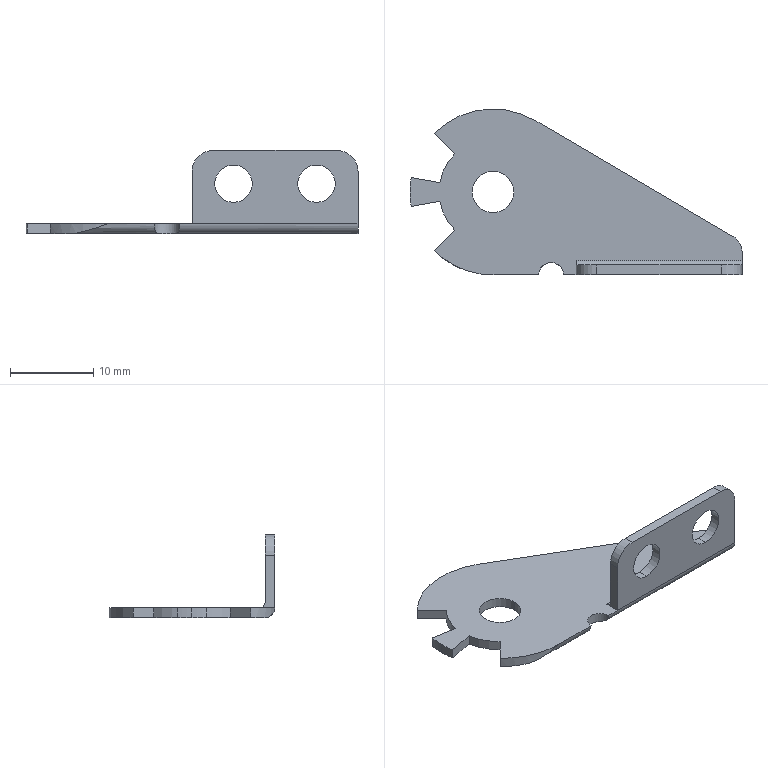Part | STEP file | 1 solid | 31 faces | box 40 x 20 x 10 mm | volume 737.758 mm3 | cylinder 19 | plane 12 | commonest cylinder face diameters 4.5 x4 5 x4 20 x4 2.4 x2 13 x2 1.2 x1